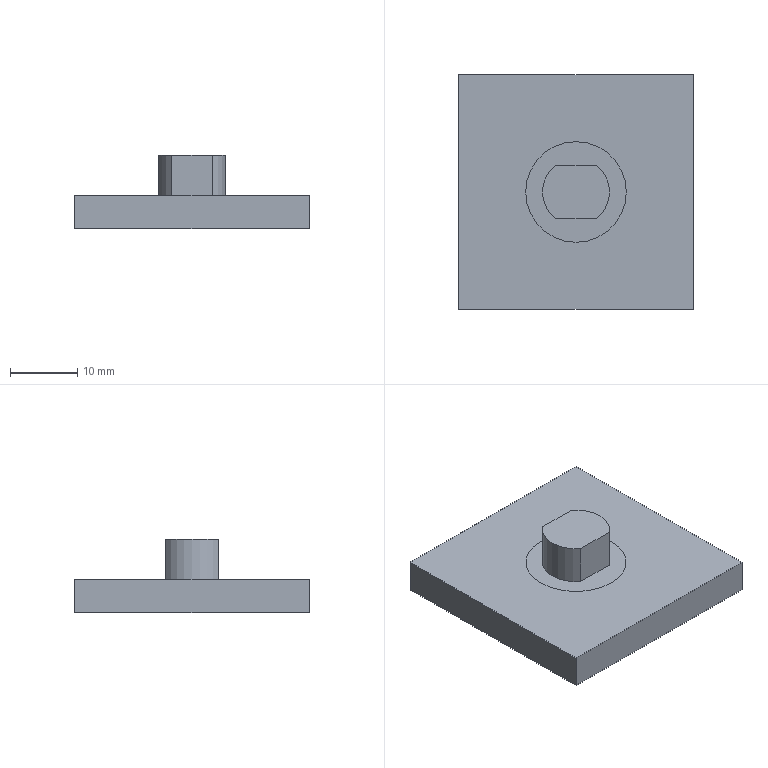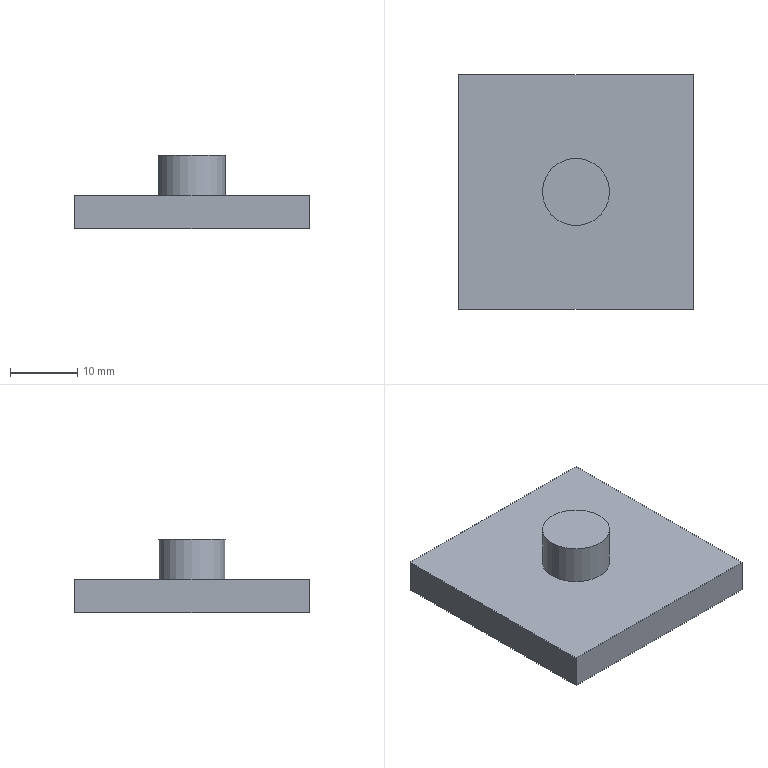CAM job | NX | 3-axis milling | part box 35 x 35 x 11 mm | stock box 35 x 35 x 11 mm
Operations:
program,operation,operation_type,tool,method,geometry_group,spindle_rpm,surface_speed,feed_per_tooth,feed_cut,feed_plunge,cut_length_mm,path_length_mm,cut_time_min,machine_time_min
1,ZLEVEL_PROFILE,ZLevelMilling,D10,METHOD,A,3000.0,94.0,0.3333,2000.0,1000.0,767.745,936.246,0.4551,0.472
1,ZLEVEL_PROFILE_COPY,ZLevelMilling,D10JING,METHOD,A,5000.0,157.0,0.1,1000.0,1000.0,26.827,191.913,0.0268,0.0433
1,PLANAR_MILL_COPY,PlanarMilling,D6A45,METHOD,A,7500.0,141.0,0.0933,1400.0,100.0,22.189,150.989,0.0158,0.0287
2,HOLE_MILLING,CylinderMilling,D10,METHOD,B,7000.0,219.0,0.1429,2000.0,100.0,110.131,174.631,0.0551,0.0615